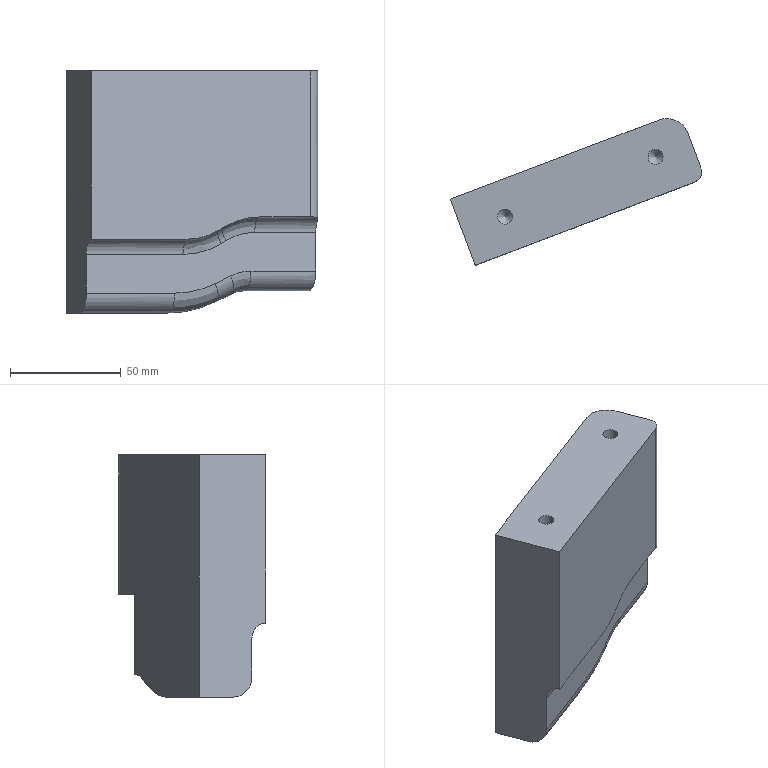Part | NX | features 8 2 | 1 solid | 31 faces | box 113.689 x 66.365 x 109.5 mm | volume 339011 mm3 | plane 11 | cylinder 11 | spline 6 | cone 3 | commonest cylinder face diameters 14 x3 18 x3 6.8 x2 8.5 x1 10 x1 20 x1